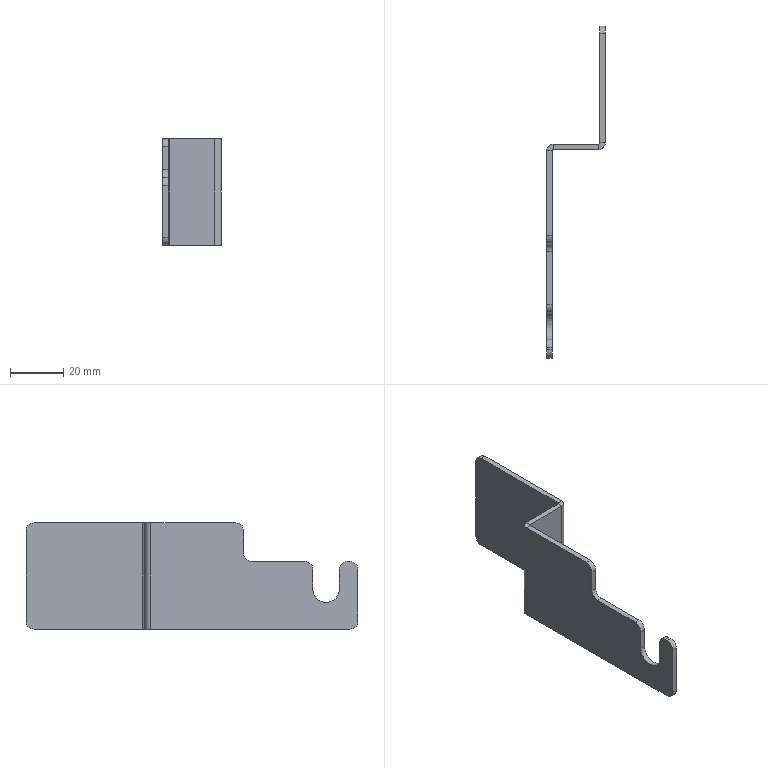Part | STEP file | 1 solid | 36 faces | box 22 x 125 x 40 mm | volume 9938 mm3 | plane 23 | cylinder 13 | commonest cylinder face diameters 6 x8 1 x2 5 x2 10 x1